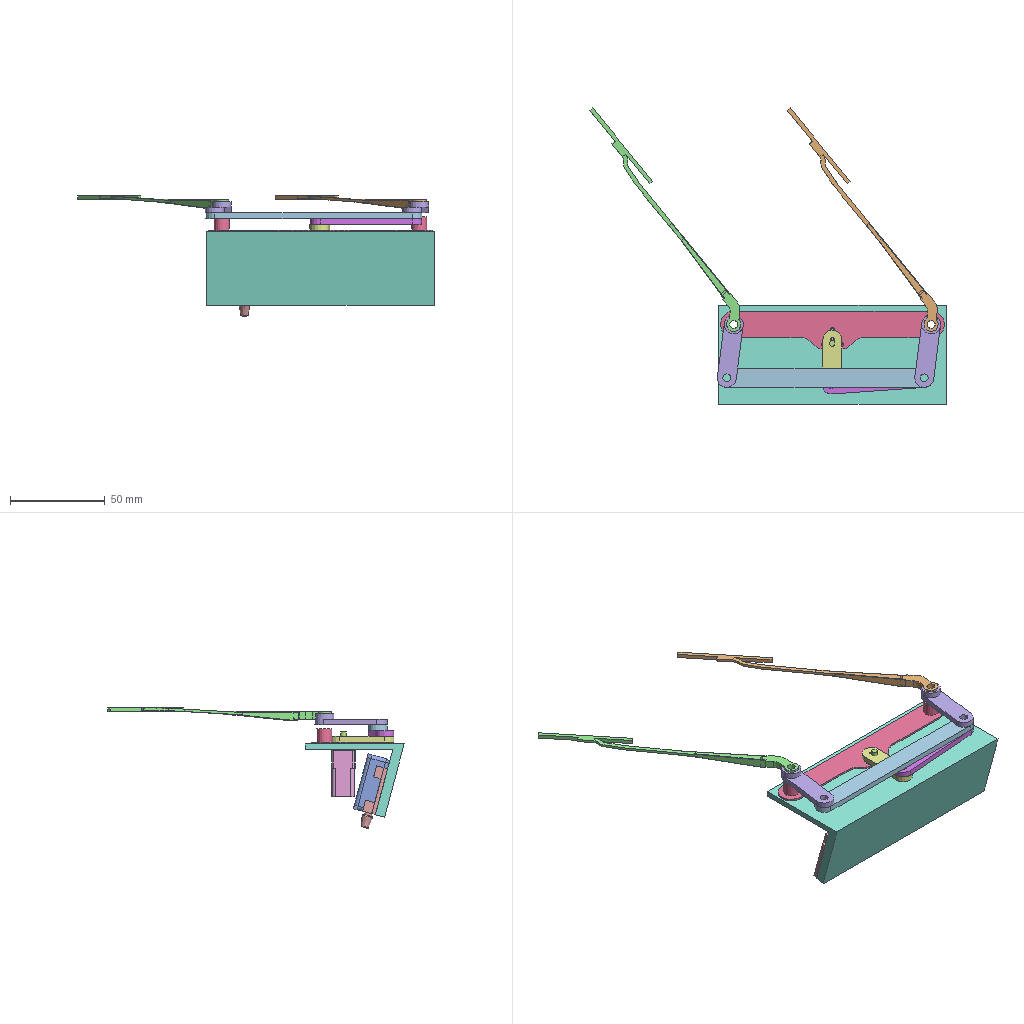Assembly | NX | 12 different items | 13 placed | box 188 x 156 x 63 mm
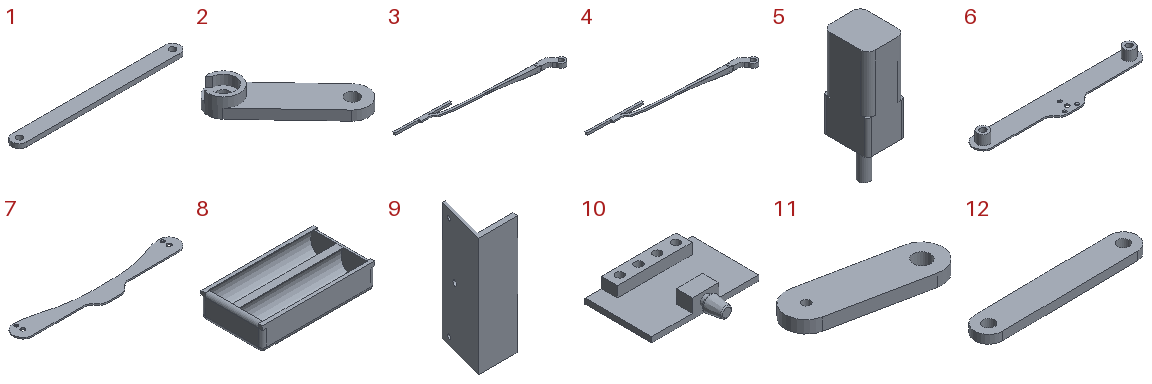Parts list (item | quantity | size | volume | features):
1 | x1 | 114 x 10 x 3 mm | 3272 mm3 | features DATUM_CSYS 2, OFFSET_REGION 2, BREP 1, EXTRUDE 1, SCALE 1, SKETCH 1
2 | x2 | 29.552 x 30.598 x 6 mm | 1085 mm3 | features DATUM_CSYS 3, EXTRUDE 2, OFFSET_REGION 2, SKETCH 2, BREP 1, SCALE 1
3 | x1 | 138.697 x 21.869 x 6.967 mm | 1173 mm3 | features DATUM_CSYS 3, OFFSET_REGION 3, BREP 2, EXTRUDE 2, SKETCH 2, SCALE 1, UNITE 1
4 | x1 | 138.697 x 21.869 x 6.967 mm | 1173 mm3 | features DATUM_CSYS 3, OFFSET_REGION 3, BREP 2, EXTRUDE 2, SKETCH 2, SCALE 1, UNITE 1
5 | x1 | 10 x 12 x 34 mm | 2897 mm3 | features DATUM_CSYS 4, EXTRUDE 4, SKETCH 3, BLEND 2, UNITE 2
6 | x1 | 118 x 20 x 8 mm | 2204 mm3 | features DATUM_CSYS 4, EXTRUDE 4, SKETCH 3, BREP 1, OFFSET_REGION 1, SCALE 1
7 | x1 | 118 x 20 x 1 mm | 1195 mm3 | features BREP 1, DATUM_CSYS 1, SCALE 1
8 | x1 | 55 x 30 x 12 mm | 6346 mm3 | features DATUM_CSYS 3, EXTRUDE 2, SKETCH 2, BLEND 1
9 | x1 | 40 x 50.228 x 120 mm | 40168 mm3 | features DATUM_CSYS 5, SKETCH 4, EXTRUDE 3, OFFSET_REGION 1
10 | x1 | 40 x 33 x 7 mm | 3005 mm3 | features DATUM_CSYS 6, EXTRUDE 5, SKETCH 5, BLEND 2, CHAMFER 1
11 | x1 | 33.164 x 14.761 x 3 mm | 894.076 mm3 | features DATUM_CSYS 2, OFFSET_REGION 2, BREP 1, EXTRUDE 1, SCALE 1, SKETCH 1
12 | x1 | 59.014 x 10.685 x 3 mm | 1623 mm3 | features DATUM_CSYS 2, OFFSET_REGION 2, BREP 1, EXTRUDE 1, SCALE 1, SKETCH 1
Mates (type | each side: item.copy, entity, surface, feature):
Fix | 8.1 component
Fix | 5.1 component
Fix | 9.1 component
Fix | 10.1 component
Concentric | 6.1 edge | 9.1 edge | 2 times
Concentric | 11.1 edge | 6.1 edge
Concentric | 12.1 edge | 11.1 edge
Concentric | 1.1 edge | 12.1 edge
Concentric | 2.1 edge | 1.1 edge | 2 times
Concentric | 3.1 edge | 2.1 edge
Concentric | 4.1 edge | 2.1 edge